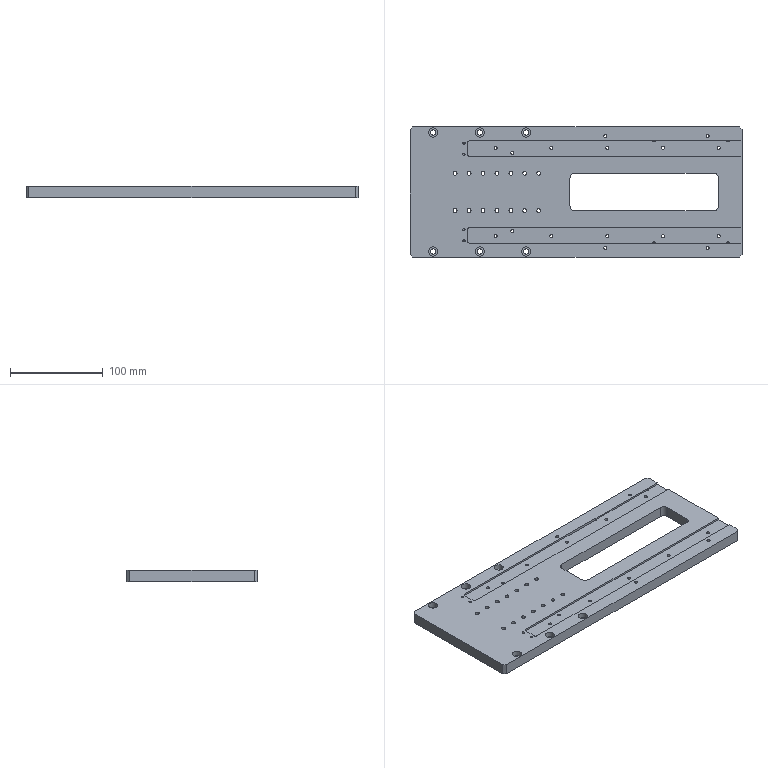NC program | NX | posted with a generic post | part box 357 x 140 x 12 mm
Lines 38 to 860 of 6551:
(ZLEVEL_PROFILE_1_1 , TOOL : D3)
N62 T16 M6
N64 G54
N66 G17 G0 G90 X-59.136 Y0.252 B0. C0. S9500 M3
N68 G43 Z30. H16
N70 Z1.5
N72 G94 G1 X-59.174 Y0.382 Z1.493 F1000.
N74 X-59.385 Y0.671 Z1.474
N76 X-59.692 Y0.856 Z1.455
N78 X-60.046 Y0.909 Z1.437
N80 X-60.394 Y0.82 Z1.418
N82 X-60.616 Y0.669 Z1.404
N84 X-60.836 Y0.36 Z1.384
N86 X-60.91 Y-0.012 Z1.364
N88 X-60.826 Y-0.381 Z1.344
N90 X-60.599 Y-0.685 Z1.324
N92 X-60.373 Y-0.83 Z1.31
N94 X-60.135 Y-0.9 Z1.297
N96 X-59.865 Z1.283
N98 X-59.564 Y-0.799 Z1.266
N100 X-59.315 Y-0.599 Z1.25
N102 X-59.17 Y-0.373 Z1.236
N104 X-59.099 Y-0.13 Z1.222
N106 X-59.098 Y0.123 Z1.209
N108 X-59.174 Y0.382 Z1.195
N110 X-59.385 Y0.671 Z1.176
N112 X-59.692 Y0.856 Z1.157
N114 X-60.046 Y0.909 Z1.139
N116 X-60.394 Y0.82 Z1.12
N118 X-60.616 Y0.669 Z1.106
N120 X-60.836 Y0.36 Z1.086
N122 X-60.91 Y-0.012 Z1.066
N124 X-60.826 Y-0.381 Z1.046
N126 X-60.599 Y-0.685 Z1.026
N128 X-60.373 Y-0.83 Z1.012
N130 X-60.135 Y-0.9 Z0.999
N132 X-59.865 Z0.985
N134 X-59.564 Y-0.799 Z0.968
N136 X-59.315 Y-0.599 Z0.952
N138 X-59.17 Y-0.373 Z0.938
N140 X-59.099 Y-0.13 Z0.924
N142 X-59.098 Y0.123 Z0.911
N144 X-59.174 Y0.382 Z0.897
N146 X-59.385 Y0.671 Z0.878
N148 X-59.692 Y0.856 Z0.859
N150 X-60.046 Y0.909 Z0.841
N152 X-60.394 Y0.82 Z0.822
N154 X-60.616 Y0.669 Z0.808
N156 X-60.836 Y0.36 Z0.788
N158 X-60.91 Y-0.012 Z0.768
N160 X-60.826 Y-0.381 Z0.748
N162 X-60.599 Y-0.685 Z0.728
N164 X-60.373 Y-0.83 Z0.714
N166 X-60.135 Y-0.9 Z0.701
N168 X-59.865 Z0.687
N170 X-59.564 Y-0.799 Z0.67
N172 X-59.315 Y-0.599 Z0.654
N174 X-59.17 Y-0.373 Z0.64
N176 X-59.099 Y-0.13 Z0.626
N178 X-59.098 Y0.123 Z0.613
N180 X-59.174 Y0.382 Z0.599
N182 X-59.385 Y0.671 Z0.58
N184 X-59.692 Y0.856 Z0.561
N186 X-60.046 Y0.909 Z0.543
N188 X-60.394 Y0.82 Z0.524
N190 X-60.616 Y0.669 Z0.51
N192 X-60.836 Y0.36 Z0.49
N194 X-60.91 Y-0.012 Z0.47
N196 X-60.826 Y-0.381 Z0.45
N198 X-60.599 Y-0.685 Z0.43
N200 X-60.373 Y-0.83 Z0.416
N202 X-60.135 Y-0.9 Z0.403
N204 X-59.865 Z0.389
N206 X-59.564 Y-0.799 Z0.372
N208 X-59.315 Y-0.599 Z0.356
N210 X-59.17 Y-0.373 Z0.341
N212 X-59.099 Y-0.13 Z0.328
N214 X-59.098 Y0.123 Z0.315
N216 X-59.174 Y0.382 Z0.301
N218 X-59.385 Y0.671 Z0.282
N220 X-59.692 Y0.856 Z0.263
N222 X-60.046 Y0.909 Z0.245
N224 X-60.394 Y0.82 Z0.226
N226 X-60.616 Y0.669 Z0.212
N228 X-60.836 Y0.36 Z0.192
N230 X-60.91 Y-0.012 Z0.172
N232 X-60.826 Y-0.381 Z0.152
N234 X-60.599 Y-0.685 Z0.132
N236 X-60.373 Y-0.83 Z0.118
N238 X-60.135 Y-0.9 Z0.105
N240 X-59.865 Z0.091
N242 X-59.564 Y-0.799 Z0.074
N244 X-59.315 Y-0.599 Z0.058
N246 X-59.17 Y-0.373 Z0.043
N248 X-59.099 Y-0.13 Z0.03
N250 X-59.098 Y0.123 Z0.017
N252 X-59.174 Y0.382 Z0.003
N254 X-59.385 Y0.671 Z-0.016
N256 X-59.692 Y0.856 Z-0.035
N258 X-60.046 Y0.909 Z-0.053
N260 X-60.394 Y0.82 Z-0.072
N262 X-60.616 Y0.669 Z-0.086
N264 X-60.836 Y0.36 Z-0.106
N266 X-60.91 Y-0.012 Z-0.126
N268 X-60.826 Y-0.381 Z-0.146
N270 X-60.599 Y-0.685 Z-0.166
N272 X-60.373 Y-0.83 Z-0.18
N274 X-60.135 Y-0.9 Z-0.193
N276 X-60. Z-0.2
N278 G3 X-59.1 Y0. R0.9 F1200.
N280 X-60. Y-0.9 R-0.9
N282 G1 X-59.878 Y-0.883 Z-0.204
N284 X-59.78 Y-0.863 Z-0.208
N286 X-59.649 Y-0.819 Z-0.213
N288 X-59.572 Y-0.784 Z-0.216
N290 X-59.471 Y-0.718 Z-0.22
N292 X-59.393 Y-0.652 Z-0.224
N294 X-59.299 Y-0.552 Z-0.229
N296 X-59.249 Y-0.482 Z-0.232
N298 X-59.181 Y-0.35 Z-0.237
N300 X-59.145 Y-0.251 Z-0.241
N302 X-59.115 Y-0.097 Z-0.247
N304 X-59.106 Y-0.001 Z-0.25
N306 X-59.113 Y0.087 Z-0.253
N308 X-59.117 Y0.131 Z-0.255
N310 X-59.123 Y0.171 Z-0.256
N312 X-59.145 Y0.25 Z-0.259
N314 X-59.201 Y0.394 Z-0.265
N316 X-59.241 Y0.469 Z-0.268
N318 X-59.293 Y0.543 Z-0.271
N320 X-59.319 Y0.579 Z-0.272
N322 X-59.344 Y0.604 Z-0.274
N324 X-59.394 Y0.653 Z-0.276
N326 X-59.512 Y0.746 Z-0.282
N328 X-59.588 Y0.791 Z-0.285
N330 X-59.718 Y0.847 Z-0.29
N332 X-59.813 Y0.872 Z-0.293
N334 X-59.95 Y0.89 Z-0.298
N336 X-60.052 Y0.889 Z-0.302
N338 X-60.196 Y0.87 Z-0.307
N340 X-60.287 Y0.846 Z-0.31
N342 X-60.408 Y0.792 Z-0.315
N344 X-60.5 Y0.737 Z-0.319
N346 X-60.621 Y0.639 Z-0.325
N348 X-60.688 Y0.571 Z-0.328
N350 X-60.739 Y0.498 Z-0.331
N352 X-60.764 Y0.462 Z-0.333
N354 X-60.783 Y0.427 Z-0.334
N356 X-60.817 Y0.356 Z-0.337
N358 X-60.853 Y0.256 Z-0.341
N360 X-60.876 Y0.175 Z-0.344
N362 X-60.885 Y0.114 Z-0.346
N364 X-60.89 Y-0.05 Z-0.352
N366 X-60.882 Y-0.137 Z-0.355
N368 X-60.849 Y-0.27 Z-0.36
N370 X-60.808 Y-0.376 Z-0.364
N372 X-60.732 Y-0.508 Z-0.369
N374 X-60.672 Y-0.588 Z-0.373
N376 X-60.606 Y-0.655 Z-0.376
N378 X-60.572 Y-0.687 Z-0.378
N380 X-60.542 Y-0.709 Z-0.379
N382 X-60.482 Y-0.751 Z-0.382
N384 X-60.353 Y-0.818 Z-0.387
N386 X-60.251 Y-0.855 Z-0.391
N388 X-60.126 Y-0.884 Z-0.395
N390 X-60. Y-0.9 Z-0.4
N392 X-59.878 Y-0.883 Z-0.404
N394 X-59.78 Y-0.863 Z-0.408
N396 X-59.649 Y-0.819 Z-0.413
N398 X-59.572 Y-0.784 Z-0.416
N400 X-59.472 Y-0.718 Z-0.42
N402 X-59.393 Y-0.652 Z-0.424
N404 X-59.299 Y-0.552 Z-0.429
N406 X-59.249 Y-0.482 Z-0.432
N408 X-59.181 Y-0.35 Z-0.437
N410 X-59.145 Y-0.251 Z-0.441
N412 X-59.115 Y-0.097 Z-0.447
N414 X-59.106 Y-0.001 Z-0.45
N416 X-59.113 Y0.087 Z-0.453
N418 X-59.117 Y0.131 Z-0.455
N420 X-59.124 Y0.171 Z-0.456
N422 X-59.145 Y0.25 Z-0.459
N424 X-59.201 Y0.394 Z-0.465
N426 X-59.241 Y0.469 Z-0.468
N428 X-59.293 Y0.543 Z-0.471
N430 X-59.319 Y0.579 Z-0.472
N432 X-59.344 Y0.604 Z-0.474
N434 X-59.394 Y0.653 Z-0.476
N436 X-59.512 Y0.746 Z-0.482
N438 X-59.588 Y0.791 Z-0.485
N440 X-59.718 Y0.847 Z-0.49
N442 X-59.813 Y0.872 Z-0.493
N444 X-59.95 Y0.89 Z-0.498
N446 X-60.052 Y0.889 Z-0.502
N448 X-60.196 Y0.87 Z-0.507
N450 X-60.287 Y0.846 Z-0.51
N452 X-60.408 Y0.792 Z-0.515
N454 X-60.5 Y0.737 Z-0.519
N456 X-60.621 Y0.639 Z-0.525
N458 X-60.688 Y0.571 Z-0.528
N460 X-60.739 Y0.498 Z-0.531
N462 X-60.764 Y0.462 Z-0.533
N464 X-60.783 Y0.427 Z-0.534
N466 X-60.817 Y0.356 Z-0.537
N468 X-60.853 Y0.256 Z-0.541
N470 X-60.876 Y0.175 Z-0.544
N472 X-60.885 Y0.114 Z-0.546
N474 X-60.89 Y-0.05 Z-0.552
N476 X-60.882 Y-0.137 Z-0.555
N478 X-60.849 Y-0.27 Z-0.56
N480 X-60.808 Y-0.376 Z-0.564
N482 X-60.732 Y-0.508 Z-0.569
N484 X-60.672 Y-0.588 Z-0.573
N486 X-60.606 Y-0.654 Z-0.576
N488 X-60.572 Y-0.687 Z-0.578
N490 X-60.542 Y-0.709 Z-0.579
N492 X-60.482 Y-0.751 Z-0.582
N494 X-60.353 Y-0.818 Z-0.587
N496 X-60.251 Y-0.855 Z-0.591
N498 X-60.126 Y-0.884 Z-0.595
N500 X-60. Y-0.9 Z-0.6
N502 X-59.878 Y-0.883 Z-0.604
N504 X-59.78 Y-0.863 Z-0.608
N506 X-59.649 Y-0.819 Z-0.613
N508 X-59.572 Y-0.784 Z-0.616
N510 X-59.472 Y-0.718 Z-0.62
N512 X-59.393 Y-0.652 Z-0.624
N514 X-59.299 Y-0.552 Z-0.629
N516 X-59.249 Y-0.482 Z-0.632
N518 X-59.181 Y-0.35 Z-0.637
N520 X-59.145 Y-0.251 Z-0.641
N522 X-59.115 Y-0.097 Z-0.647
N524 X-59.106 Y-0.001 Z-0.65
N526 X-59.113 Y0.087 Z-0.653
N528 X-59.117 Y0.131 Z-0.655
N530 X-59.124 Y0.171 Z-0.656
N532 X-59.145 Y0.25 Z-0.659
N534 X-59.201 Y0.394 Z-0.665
N536 X-59.241 Y0.469 Z-0.668
N538 X-59.293 Y0.542 Z-0.671
N540 X-59.319 Y0.579 Z-0.672
N542 X-59.344 Y0.604 Z-0.674
N544 X-59.394 Y0.653 Z-0.676
N546 X-59.512 Y0.746 Z-0.682
N548 X-59.588 Y0.791 Z-0.685
N550 X-59.718 Y0.847 Z-0.69
N552 X-59.813 Y0.872 Z-0.693
N554 X-59.95 Y0.889 Z-0.698
N556 X-60.052 Z-0.702
N558 X-60.196 Y0.87 Z-0.707
N560 X-60.287 Y0.846 Z-0.71
N562 X-60.408 Y0.792 Z-0.715
N564 X-60.5 Y0.737 Z-0.719
N566 X-60.621 Y0.639 Z-0.725
N568 X-60.688 Y0.571 Z-0.728
N570 X-60.739 Y0.498 Z-0.731
N572 X-60.764 Y0.462 Z-0.733
N574 X-60.783 Y0.427 Z-0.734
N576 X-60.817 Y0.356 Z-0.737
N578 X-60.853 Y0.256 Z-0.741
N580 X-60.876 Y0.175 Z-0.744
N582 X-60.885 Y0.114 Z-0.746
N584 X-60.889 Y-0.05 Z-0.752
N586 X-60.882 Y-0.137 Z-0.755
N588 X-60.849 Y-0.27 Z-0.76
N590 X-60.808 Y-0.376 Z-0.764
N592 X-60.732 Y-0.508 Z-0.769
N594 X-60.672 Y-0.588 Z-0.773
N596 X-60.606 Y-0.654 Z-0.776
N598 X-60.572 Y-0.687 Z-0.778
N600 X-60.542 Y-0.709 Z-0.779
N602 X-60.482 Y-0.751 Z-0.782
N604 X-60.354 Y-0.818 Z-0.787
N606 X-60.251 Y-0.855 Z-0.791
N608 X-60.126 Y-0.884 Z-0.795
N610 X-60. Y-0.9 Z-0.8
N612 X-59.879 Y-0.883 Z-0.804
N614 X-59.78 Y-0.863 Z-0.808
N616 X-59.649 Y-0.819 Z-0.813
N618 X-59.572 Y-0.784 Z-0.816
N620 X-59.472 Y-0.718 Z-0.82
N622 X-59.393 Y-0.652 Z-0.824
N624 X-59.299 Y-0.552 Z-0.829
N626 X-59.249 Y-0.482 Z-0.832
N628 X-59.181 Y-0.35 Z-0.837
N630 X-59.145 Y-0.251 Z-0.841
N632 X-59.115 Y-0.097 Z-0.847
N634 X-59.106 Y-0.001 Z-0.85
N636 X-59.113 Y0.087 Z-0.853
N638 X-59.117 Y0.131 Z-0.855
N640 X-59.124 Y0.171 Z-0.856
N642 X-59.145 Y0.25 Z-0.859
N644 X-59.201 Y0.394 Z-0.865
N646 X-59.241 Y0.469 Z-0.868
N648 X-59.293 Y0.545 Z-0.871
N650 X-59.321 Y0.581 Z-0.873
N652 X-59.345 Y0.605 Z-0.874
N654 X-59.394 Y0.653 Z-0.876
N656 X-59.513 Y0.747 Z-0.882
N658 X-59.588 Y0.791 Z-0.885
N660 X-59.718 Y0.847 Z-0.89
N662 X-59.813 Y0.872 Z-0.893
N664 X-59.95 Y0.889 Z-0.898
N666 X-60.052 Z-0.902
N668 X-60.196 Y0.87 Z-0.907
N670 X-60.287 Y0.846 Z-0.91
N672 X-60.408 Y0.792 Z-0.915
N674 X-60.5 Y0.737 Z-0.919
N676 X-60.621 Y0.639 Z-0.925
N678 X-60.688 Y0.571 Z-0.928
N680 X-60.739 Y0.498 Z-0.931
N682 X-60.764 Y0.462 Z-0.933
N684 X-60.783 Y0.427 Z-0.934
N686 X-60.817 Y0.356 Z-0.937
N688 X-60.853 Y0.256 Z-0.941
N690 X-60.875 Y0.176 Z-0.944
N692 X-60.885 Y0.114 Z-0.946
N694 X-60.889 Y-0.05 Z-0.952
N696 X-60.882 Y-0.137 Z-0.955
N698 X-60.849 Y-0.27 Z-0.96
N700 X-60.808 Y-0.376 Z-0.964
N702 X-60.732 Y-0.508 Z-0.969
N704 X-60.672 Y-0.588 Z-0.973
N706 X-60.606 Y-0.654 Z-0.976
N708 X-60.572 Y-0.687 Z-0.978
N710 X-60.542 Y-0.709 Z-0.979
N712 X-60.482 Y-0.751 Z-0.982
N714 X-60.354 Y-0.818 Z-0.987
N716 X-60.251 Y-0.855 Z-0.991
N718 X-60.126 Y-0.883 Z-0.995
N720 X-60. Y-0.9 Z-1.
N722 X-59.879 Y-0.883 Z-1.004
N724 X-59.78 Y-0.863 Z-1.008
N726 X-59.649 Y-0.819 Z-1.013
N728 X-59.572 Y-0.783 Z-1.016
N730 X-59.472 Y-0.718 Z-1.02
N732 X-59.393 Y-0.652 Z-1.024
N734 X-59.299 Y-0.552 Z-1.029
N736 X-59.249 Y-0.482 Z-1.032
N738 X-59.181 Y-0.35 Z-1.037
N740 X-59.145 Y-0.251 Z-1.041
N742 X-59.115 Y-0.097 Z-1.047
N744 X-59.106 Y-0.001 Z-1.05
N746 X-59.113 Y0.087 Z-1.053
N748 X-59.117 Y0.131 Z-1.055
N750 X-59.124 Y0.171 Z-1.056
N752 X-59.145 Y0.25 Z-1.059
N754 X-59.201 Y0.394 Z-1.065
N756 X-59.241 Y0.469 Z-1.068
N758 X-59.293 Y0.545 Z-1.071
N760 X-59.321 Y0.581 Z-1.073
N762 X-59.345 Y0.605 Z-1.074
N764 X-59.394 Y0.653 Z-1.076
N766 X-59.513 Y0.746 Z-1.082
N768 X-59.588 Y0.791 Z-1.085
N770 X-59.718 Y0.847 Z-1.09
N772 X-59.813 Y0.872 Z-1.093
N774 X-59.95 Y0.889 Z-1.098
N776 X-60.052 Z-1.102
N778 X-60.196 Y0.87 Z-1.107
N780 X-60.287 Y0.846 Z-1.11
N782 X-60.408 Y0.792 Z-1.115
N784 X-60.5 Y0.737 Z-1.119
N786 X-60.621 Y0.639 Z-1.125
N788 X-60.688 Y0.571 Z-1.128
N790 X-60.739 Y0.498 Z-1.131
N792 X-60.764 Y0.462 Z-1.133
N794 X-60.783 Y0.427 Z-1.134
N796 X-60.817 Y0.356 Z-1.137
N798 X-60.867 Y0.205 Z-1.143
N800 X-60.885 Y0.114 Z-1.146
N802 X-60.891 Y-0.037 Z-1.151
N804 X-60.882 Y-0.137 Z-1.155
N806 X-60.849 Y-0.27 Z-1.16
N808 X-60.808 Y-0.376 Z-1.164
N810 X-60.732 Y-0.508 Z-1.169
N812 X-60.672 Y-0.587 Z-1.173
N814 X-60.606 Y-0.654 Z-1.176
N816 X-60.572 Y-0.687 Z-1.178
N818 X-60.542 Y-0.709 Z-1.179
N820 X-60.482 Y-0.751 Z-1.182
N822 X-60.354 Y-0.817 Z-1.187
N824 X-60.251 Y-0.855 Z-1.191
N826 X-60.126 Y-0.883 Z-1.195
N828 X-60. Y-0.9 Z-1.2
N830 X-59.879 Y-0.883 Z-1.204
N832 X-59.78 Y-0.863 Z-1.208
N834 X-59.649 Y-0.819 Z-1.213
N836 X-59.572 Y-0.783 Z-1.216
N838 X-59.472 Y-0.718 Z-1.22
N840 X-59.393 Y-0.652 Z-1.224
N842 X-59.299 Y-0.552 Z-1.229
N844 X-59.249 Y-0.482 Z-1.232
N846 X-59.181 Y-0.35 Z-1.237
N848 X-59.145 Y-0.251 Z-1.241
N850 X-59.115 Y-0.098 Z-1.247
N852 X-59.106 Y-0.001 Z-1.25
N854 X-59.113 Y0.087 Z-1.253
N856 X-59.117 Y0.131 Z-1.255
N858 X-59.124 Y0.171 Z-1.256
N860 X-59.145 Y0.25 Z-1.259
N862 X-59.2 Y0.394 Z-1.265
N864 X-59.241 Y0.469 Z-1.268
N866 X-59.293 Y0.545 Z-1.271
N868 X-59.321 Y0.581 Z-1.273
N870 X-59.345 Y0.605 Z-1.274
N872 X-59.394 Y0.653 Z-1.276
N874 X-59.513 Y0.746 Z-1.282
N876 X-59.588 Y0.791 Z-1.285
N878 X-59.718 Y0.847 Z-1.29
N880 X-59.813 Y0.872 Z-1.293
N882 X-59.95 Y0.889 Z-1.298
N884 X-60.052 Z-1.302
N886 X-60.196 Y0.87 Z-1.307
N888 X-60.287 Y0.846 Z-1.31
N890 X-60.408 Y0.792 Z-1.315
N892 X-60.5 Y0.737 Z-1.319
N894 X-60.621 Y0.639 Z-1.325
N896 X-60.688 Y0.571 Z-1.328
N898 X-60.739 Y0.499 Z-1.331
N900 X-60.764 Y0.462 Z-1.333
N902 X-60.783 Y0.427 Z-1.334
N904 X-60.817 Y0.356 Z-1.337
N906 X-60.867 Y0.206 Z-1.343
N908 X-60.885 Y0.114 Z-1.346
N910 X-60.891 Y-0.037 Z-1.351
N912 X-60.882 Y-0.137 Z-1.355
N914 X-60.849 Y-0.27 Z-1.36
N916 X-60.808 Y-0.376 Z-1.364
N918 X-60.732 Y-0.508 Z-1.369
N920 X-60.672 Y-0.587 Z-1.373
N922 X-60.606 Y-0.654 Z-1.376
N924 X-60.572 Y-0.687 Z-1.378
N926 X-60.542 Y-0.708 Z-1.379
N928 X-60.482 Y-0.751 Z-1.382
N930 X-60.354 Y-0.817 Z-1.387
N932 X-60.251 Y-0.855 Z-1.391
N934 X-60.126 Y-0.883 Z-1.395
N936 X-60. Y-0.9 Z-1.4
N938 X-59.879 Y-0.883 Z-1.404
N940 X-59.78 Y-0.863 Z-1.408
N942 X-59.65 Y-0.819 Z-1.413
N944 X-59.572 Y-0.783 Z-1.416
N946 X-59.472 Y-0.718 Z-1.42
N948 X-59.393 Y-0.652 Z-1.424
N950 X-59.299 Y-0.552 Z-1.429
N952 X-59.249 Y-0.482 Z-1.432
N954 X-59.181 Y-0.35 Z-1.437
N956 X-59.145 Y-0.251 Z-1.441
N958 X-59.115 Y-0.098 Z-1.447
N960 X-59.106 Y-0.001 Z-1.45
N962 X-59.113 Y0.087 Z-1.453
N964 X-59.117 Y0.131 Z-1.455
N966 X-59.124 Y0.171 Z-1.456
N968 X-59.145 Y0.25 Z-1.459
N970 X-59.2 Y0.394 Z-1.465
N972 X-59.241 Y0.469 Z-1.468
N974 X-59.293 Y0.545 Z-1.471
N976 X-59.321 Y0.581 Z-1.473
N978 X-59.345 Y0.605 Z-1.474
N980 X-59.394 Y0.653 Z-1.476
N982 X-59.513 Y0.746 Z-1.482
N984 X-59.588 Y0.791 Z-1.485
N986 X-59.718 Y0.847 Z-1.49
N988 X-59.813 Y0.872 Z-1.493
N990 X-59.95 Y0.889 Z-1.498
N992 X-60.052 Z-1.502
N994 X-60.196 Y0.87 Z-1.507
N996 X-60.287 Y0.846 Z-1.51
N998 X-60.408 Y0.792 Z-1.515
N1000 X-60.5 Y0.737 Z-1.519
N1002 X-60.621 Y0.639 Z-1.525
N1004 X-60.688 Y0.571 Z-1.528
N1006 X-60.739 Y0.499 Z-1.531
N1008 X-60.764 Y0.462 Z-1.533
N1010 X-60.783 Y0.428 Z-1.534
N1012 X-60.817 Y0.356 Z-1.537
N1014 X-60.867 Y0.206 Z-1.543
N1016 X-60.884 Y0.114 Z-1.546
N1018 X-60.891 Y-0.037 Z-1.551
N1020 X-60.882 Y-0.137 Z-1.555
N1022 X-60.849 Y-0.27 Z-1.56
N1024 X-60.808 Y-0.376 Z-1.564
N1026 X-60.732 Y-0.507 Z-1.569
N1028 X-60.672 Y-0.587 Z-1.573
N1030 X-60.606 Y-0.654 Z-1.576
N1032 X-60.572 Y-0.687 Z-1.578
N1034 X-60.542 Y-0.708 Z-1.579
N1036 X-60.482 Y-0.751 Z-1.582
N1038 X-60.398 Y-0.798 Z-1.585
N1040 X-60.321 Y-0.834 Z-1.588
N1042 X-60.251 Y-0.855 Z-1.591
N1044 X-60.126 Y-0.883 Z-1.595
N1046 X-60. Y-0.9 Z-1.6
N1048 X-59.879 Y-0.883 Z-1.604
N1050 X-59.78 Y-0.863 Z-1.608
N1052 X-59.65 Y-0.819 Z-1.613
N1054 X-59.572 Y-0.783 Z-1.616
N1056 X-59.472 Y-0.718 Z-1.62
N1058 X-59.393 Y-0.652 Z-1.624
N1060 X-59.299 Y-0.552 Z-1.629
N1062 X-59.249 Y-0.482 Z-1.632
N1064 X-59.181 Y-0.35 Z-1.637
N1066 X-59.145 Y-0.251 Z-1.641
N1068 X-59.115 Y-0.098 Z-1.646
N1070 X-59.106 Y-0.001 Z-1.65
N1072 X-59.113 Y0.087 Z-1.653
N1074 X-59.117 Y0.131 Z-1.655
N1076 X-59.124 Y0.171 Z-1.656
N1078 X-59.145 Y0.25 Z-1.659
N1080 X-59.2 Y0.394 Z-1.665
N1082 X-59.241 Y0.469 Z-1.668
N1084 X-59.293 Y0.544 Z-1.671
N1086 X-59.321 Y0.581 Z-1.673
N1088 X-59.345 Y0.605 Z-1.674
N1090 X-59.394 Y0.653 Z-1.676
N1092 X-59.513 Y0.746 Z-1.682
N1094 X-59.588 Y0.791 Z-1.685
N1096 X-59.718 Y0.847 Z-1.69
N1098 X-59.813 Y0.872 Z-1.693
N1100 X-59.95 Y0.89 Z-1.698
N1102 X-60.052 Y0.889 Z-1.702
N1104 X-60.198 Y0.869 Z-1.707
N1106 X-60.287 Y0.846 Z-1.71
N1108 X-60.408 Y0.792 Z-1.715
N1110 X-60.5 Y0.737 Z-1.719
N1112 X-60.621 Y0.639 Z-1.725
N1114 X-60.688 Y0.571 Z-1.728
N1116 X-60.739 Y0.499 Z-1.731
N1118 X-60.764 Y0.462 Z-1.733
N1120 X-60.783 Y0.428 Z-1.734
N1122 X-60.817 Y0.356 Z-1.737
N1124 X-60.867 Y0.206 Z-1.743
N1126 X-60.884 Y0.114 Z-1.746
N1128 X-60.89 Y-0.037 Z-1.751
N1130 X-60.882 Y-0.137 Z-1.755
N1132 X-60.849 Y-0.27 Z-1.76
N1134 X-60.807 Y-0.376 Z-1.764
N1136 X-60.732 Y-0.507 Z-1.769
N1138 X-60.672 Y-0.587 Z-1.773
N1140 X-60.606 Y-0.654 Z-1.776
N1142 X-60.572 Y-0.687 Z-1.778
N1144 X-60.542 Y-0.708 Z-1.779
N1146 X-60.482 Y-0.751 Z-1.782
N1148 X-60.398 Y-0.797 Z-1.785
N1150 X-60.321 Y-0.833 Z-1.788
N1152 X-60.251 Y-0.855 Z-1.791
N1154 X-60.126 Y-0.883 Z-1.795
N1156 X-60. Y-0.9 Z-1.8
N1158 X-59.879 Y-0.883 Z-1.804
N1160 X-59.78 Y-0.863 Z-1.808
N1162 X-59.65 Y-0.819 Z-1.813
N1164 X-59.572 Y-0.783 Z-1.816
N1166 X-59.472 Y-0.718 Z-1.82
N1168 X-59.393 Y-0.652 Z-1.824
N1170 X-59.3 Y-0.552 Z-1.829
N1172 X-59.249 Y-0.482 Z-1.832
N1174 X-59.201 Y-0.395 Z-1.835
N1176 X-59.166 Y-0.318 Z-1.838
N1178 X-59.145 Y-0.251 Z-1.841
N1180 X-59.114 Y-0.082 Z-1.847
N1182 X-59.106 Y-0.001 Z-1.85
N1184 X-59.113 Y0.087 Z-1.853
N1186 X-59.117 Y0.131 Z-1.855
N1188 X-59.124 Y0.171 Z-1.856
N1190 X-59.145 Y0.25 Z-1.859
N1192 X-59.2 Y0.394 Z-1.865
N1194 X-59.241 Y0.469 Z-1.868
N1196 X-59.293 Y0.544 Z-1.871
N1198 X-59.321 Y0.581 Z-1.873
N1200 X-59.345 Y0.605 Z-1.874
N1202 X-59.394 Y0.653 Z-1.876
N1204 X-59.513 Y0.746 Z-1.882
N1206 X-59.588 Y0.791 Z-1.885
N1208 X-59.718 Y0.846 Z-1.89
N1210 X-59.813 Y0.872 Z-1.893
N1212 X-59.95 Y0.89 Z-1.898
N1214 X-60.052 Y0.889 Z-1.902
N1216 X-60.198 Y0.869 Z-1.907
N1218 X-60.287 Y0.845 Z-1.91
N1220 X-60.408 Y0.792 Z-1.915
N1222 X-60.5 Y0.737 Z-1.919
N1224 X-60.62 Y0.639 Z-1.925
N1226 X-60.688 Y0.571 Z-1.928
N1228 X-60.739 Y0.499 Z-1.931
N1230 X-60.764 Y0.462 Z-1.933
N1232 X-60.783 Y0.428 Z-1.934
N1234 X-60.817 Y0.356 Z-1.937
N1236 X-60.867 Y0.206 Z-1.943
N1238 X-60.884 Y0.114 Z-1.946
N1240 X-60.89 Y-0.037 Z-1.951
N1242 X-60.882 Y-0.137 Z-1.955
N1244 X-60.849 Y-0.27 Z-1.96
N1246 X-60.807 Y-0.376 Z-1.964
N1248 X-60.732 Y-0.507 Z-1.969
N1250 X-60.672 Y-0.587 Z-1.973
N1252 X-60.606 Y-0.654 Z-1.976
N1254 X-60.572 Y-0.687 Z-1.978
N1256 X-60.542 Y-0.708 Z-1.979
N1258 X-60.482 Y-0.751 Z-1.982
N1260 X-60.398 Y-0.797 Z-1.985
N1262 X-60.321 Y-0.833 Z-1.988
N1264 X-60.251 Y-0.855 Z-1.991
N1266 X-60.126 Y-0.883 Z-1.995
N1268 X-60. Y-0.9 Z-2.
N1270 X-59.879 Y-0.883 Z-2.004
N1272 X-59.78 Y-0.863 Z-2.008
N1274 X-59.65 Y-0.819 Z-2.013
N1276 X-59.572 Y-0.783 Z-2.016
N1278 X-59.472 Y-0.718 Z-2.02
N1280 X-59.393 Y-0.652 Z-2.024
N1282 X-59.3 Y-0.552 Z-2.029
N1284 X-59.249 Y-0.482 Z-2.032
N1286 X-59.201 Y-0.395 Z-2.035
N1288 X-59.165 Y-0.319 Z-2.038
N1290 X-59.145 Y-0.251 Z-2.041
N1292 X-59.113 Y-0.077 Z-2.047
N1294 X-59.106 Y-0.001 Z-2.05
N1296 X-59.113 Y0.087 Z-2.053
N1298 X-59.117 Y0.132 Z-2.055
N1300 X-59.124 Y0.171 Z-2.056
N1302 X-59.145 Y0.25 Z-2.059
N1304 X-59.201 Y0.394 Z-2.065
N1306 X-59.241 Y0.469 Z-2.068
N1308 X-59.293 Y0.544 Z-2.071
N1310 X-59.321 Y0.581 Z-2.073
N1312 X-59.345 Y0.605 Z-2.074
N1314 X-59.394 Y0.653 Z-2.076
N1316 X-59.513 Y0.746 Z-2.082
N1318 X-59.588 Y0.791 Z-2.085
N1320 X-59.718 Y0.846 Z-2.09
N1322 X-59.813 Y0.872 Z-2.093
N1324 X-59.95 Y0.89 Z-2.098
N1326 X-60.052 Y0.889 Z-2.102
N1328 X-60.198 Y0.869 Z-2.107
N1330 X-60.287 Y0.845 Z-2.11
N1332 X-60.408 Y0.792 Z-2.115
N1334 X-60.5 Y0.737 Z-2.119
N1336 X-60.62 Y0.639 Z-2.125
N1338 X-60.688 Y0.571 Z-2.128
N1340 X-60.738 Y0.499 Z-2.131
N1342 X-60.764 Y0.462 Z-2.133
N1344 X-60.784 Y0.428 Z-2.134
N1346 X-60.817 Y0.356 Z-2.137
N1348 X-60.868 Y0.202 Z-2.143
N1350 X-60.884 Y0.114 Z-2.146
N1352 X-60.89 Y-0.038 Z-2.151
N1354 X-60.882 Y-0.137 Z-2.155
N1356 X-60.862 Y-0.226 Z-2.158
N1358 X-60.839 Y-0.307 Z-2.161
N1360 X-60.807 Y-0.376 Z-2.164
N1362 X-60.721 Y-0.523 Z-2.17
N1364 X-60.672 Y-0.587 Z-2.173
N1366 X-60.605 Y-0.655 Z-2.176
N1368 X-60.571 Y-0.688 Z-2.178
N1370 X-60.541 Y-0.709 Z-2.179
N1372 X-60.482 Y-0.751 Z-2.182
N1374 X-60.398 Y-0.797 Z-2.185
N1376 X-60.321 Y-0.833 Z-2.188
N1378 X-60.251 Y-0.855 Z-2.191
N1380 X-60.126 Y-0.883 Z-2.195
N1382 X-60. Y-0.9 Z-2.2
N1384 X-59.879 Y-0.883 Z-2.204
N1386 X-59.78 Y-0.863 Z-2.208
N1388 X-59.65 Y-0.819 Z-2.213
N1390 X-59.572 Y-0.783 Z-2.216
N1392 X-59.472 Y-0.718 Z-2.22
N1394 X-59.393 Y-0.652 Z-2.224
N1396 X-59.3 Y-0.552 Z-2.229
N1398 X-59.249 Y-0.482 Z-2.232
N1400 X-59.201 Y-0.395 Z-2.235
N1402 X-59.165 Y-0.319 Z-2.238
N1404 X-59.145 Y-0.251 Z-2.241
N1406 X-59.113 Y-0.077 Z-2.247
N1408 X-59.106 Y-0.001 Z-2.25
N1410 X-59.113 Y0.087 Z-2.253
N1412 X-59.117 Y0.131 Z-2.255
N1414 X-59.124 Y0.171 Z-2.256
N1416 X-59.145 Y0.25 Z-2.259
N1418 X-59.201 Y0.394 Z-2.265
N1420 X-59.241 Y0.469 Z-2.268
N1422 X-59.293 Y0.544 Z-2.271
N1424 X-59.321 Y0.581 Z-2.273
N1426 X-59.345 Y0.605 Z-2.274
N1428 X-59.394 Y0.653 Z-2.276
N1430 X-59.512 Y0.746 Z-2.282
N1432 X-59.588 Y0.791 Z-2.285
N1434 X-59.718 Y0.846 Z-2.29
N1436 X-59.813 Y0.872 Z-2.293
N1438 X-59.95 Y0.89 Z-2.298
N1440 X-60.052 Y0.889 Z-2.302
N1442 X-60.198 Y0.869 Z-2.307
N1444 X-60.287 Y0.845 Z-2.31
N1446 X-60.408 Y0.792 Z-2.315
N1448 X-60.5 Y0.737 Z-2.319
N1450 X-60.62 Y0.639 Z-2.325
N1452 X-60.688 Y0.571 Z-2.328
N1454 X-60.738 Y0.499 Z-2.331
N1456 X-60.764 Y0.462 Z-2.333
N1458 X-60.784 Y0.428 Z-2.334
N1460 X-60.817 Y0.356 Z-2.337
N1462 X-60.868 Y0.202 Z-2.343
N1464 X-60.884 Y0.114 Z-2.346
N1466 X-60.89 Y-0.038 Z-2.351
N1468 X-60.882 Y-0.137 Z-2.355
N1470 X-60.862 Y-0.226 Z-2.358
N1472 X-60.839 Y-0.307 Z-2.361
N1474 X-60.807 Y-0.376 Z-2.364
N1476 X-60.721 Y-0.523 Z-2.37
N1478 X-60.672 Y-0.587 Z-2.373
N1480 X-60.605 Y-0.655 Z-2.376
N1482 X-60.571 Y-0.688 Z-2.378
N1484 X-60.541 Y-0.709 Z-2.379
N1486 X-60.482 Y-0.751 Z-2.382
N1488 X-60.398 Y-0.797 Z-2.385
N1490 X-60.321 Y-0.833 Z-2.388
N1492 X-60.251 Y-0.855 Z-2.391
N1494 X-60.126 Y-0.883 Z-2.395
N1496 X-60. Y-0.9 Z-2.4
N1498 X-59.879 Y-0.883 Z-2.404
N1500 X-59.78 Y-0.863 Z-2.408
N1502 X-59.65 Y-0.819 Z-2.413
N1504 X-59.572 Y-0.783 Z-2.416
N1506 X-59.472 Y-0.718 Z-2.42
N1508 X-59.393 Y-0.652 Z-2.424
N1510 X-59.3 Y-0.552 Z-2.429
N1512 X-59.249 Y-0.482 Z-2.432
N1514 X-59.202 Y-0.395 Z-2.435
N1516 X-59.165 Y-0.319 Z-2.438
N1518 X-59.145 Y-0.251 Z-2.441
N1520 X-59.113 Y-0.077 Z-2.447
N1522 X-59.106 Y-0.001 Z-2.45
N1524 X-59.113 Y0.087 Z-2.453
N1526 X-59.117 Y0.131 Z-2.455
N1528 X-59.124 Y0.171 Z-2.456
N1530 X-59.145 Y0.25 Z-2.459
N1532 X-59.201 Y0.394 Z-2.465
N1534 X-59.241 Y0.469 Z-2.468
N1536 X-59.293 Y0.544 Z-2.471
N1538 X-59.321 Y0.581 Z-2.473
N1540 X-59.345 Y0.605 Z-2.474
N1542 X-59.394 Y0.653 Z-2.476
N1544 X-59.512 Y0.746 Z-2.482
N1546 X-59.588 Y0.791 Z-2.485
N1548 X-59.718 Y0.846 Z-2.49
N1550 X-59.813 Y0.872 Z-2.493
N1552 X-59.95 Y0.89 Z-2.498
N1554 X-60.052 Y0.889 Z-2.502
N1556 X-60.198 Y0.869 Z-2.507
N1558 X-60.287 Y0.845 Z-2.51
N1560 X-60.408 Y0.792 Z-2.515
N1562 X-60.5 Y0.737 Z-2.519
N1564 X-60.62 Y0.639 Z-2.525
N1566 X-60.688 Y0.571 Z-2.528
N1568 X-60.738 Y0.499 Z-2.531
N1570 X-60.764 Y0.462 Z-2.533
N1572 X-60.784 Y0.428 Z-2.534
N1574 X-60.817 Y0.356 Z-2.537
N1576 X-60.868 Y0.202 Z-2.543
N1578 X-60.884 Y0.114 Z-2.546
N1580 X-60.89 Y-0.038 Z-2.551
N1582 X-60.882 Y-0.137 Z-2.555
N1584 X-60.862 Y-0.226 Z-2.558
N1586 X-60.839 Y-0.307 Z-2.561
N1588 X-60.807 Y-0.376 Z-2.564
N1590 X-60.721 Y-0.523 Z-2.57
N1592 X-60.672 Y-0.587 Z-2.573
N1594 X-60.605 Y-0.654 Z-2.576
N1596 X-60.571 Y-0.687 Z-2.578
N1598 X-60.541 Y-0.709 Z-2.579
N1600 X-60.482 Y-0.751 Z-2.582
N1602 X-60.398 Y-0.797 Z-2.585
N1604 X-60.321 Y-0.833 Z-2.588
N1606 X-60.251 Y-0.855 Z-2.591
N1608 X-60.126 Y-0.883 Z-2.595
N1610 X-60. Y-0.9 Z-2.6
N1612 X-59.879 Y-0.883 Z-2.604
N1614 X-59.78 Y-0.863 Z-2.608
N1616 X-59.65 Y-0.819 Z-2.613
N1618 X-59.572 Y-0.783 Z-2.616
N1620 X-59.472 Y-0.718 Z-2.62
N1622 X-59.393 Y-0.652 Z-2.624
N1624 X-59.3 Y-0.553 Z-2.629
N1626 X-59.249 Y-0.482 Z-2.632
N1628 X-59.202 Y-0.395 Z-2.635
N1630 X-59.166 Y-0.319 Z-2.638
N1632 X-59.145 Y-0.251 Z-2.641
N1634 X-59.113 Y-0.078 Z-2.647
N1636 X-59.106 Y-0.001 Z-2.65
N1638 X-59.113 Y0.087 Z-2.653
N1640 X-59.117 Y0.131 Z-2.655
N1642 X-59.124 Y0.171 Z-2.656
N1644 X-59.145 Y0.25 Z-2.659
N1646 X-59.201 Y0.394 Z-2.665
N1648 X-59.241 Y0.469 Z-2.668
N1650 X-59.293 Y0.544 Z-2.671
N1652 X-59.321 Y0.581 Z-2.673
N1654 X-59.345 Y0.605 Z-2.674
N1656 X-59.394 Y0.653 Z-2.676
N1658 X-59.512 Y0.746 Z-2.682
N1660 X-59.588 Y0.791 Z-2.685
N1662 X-59.718 Y0.846 Z-2.69
N1664 X-59.813 Y0.872 Z-2.693
N1666 X-59.95 Y0.89 Z-2.698
N1668 X-60.052 Y0.889 Z-2.702
N1670 X-60.198 Y0.869 Z-2.707
N1672 X-60.287 Y0.845 Z-2.71
N1674 X-60.408 Y0.792 Z-2.715
N1676 X-60.5 Y0.737 Z-2.719
N1678 X-60.62 Y0.639 Z-2.725
N1680 X-60.688 Y0.571 Z-2.728
N1682 X-60.738 Y0.499 Z-2.731
N1684 X-60.763 Y0.462 Z-2.733
N1686 X-60.784 Y0.428 Z-2.734
N1688 X-60.817 Y0.356 Z-2.737
N1690 X-60.868 Y0.202 Z-2.743
N1692 X-60.884 Y0.114 Z-2.746
N1694 X-60.89 Y-0.038 Z-2.751
N1696 X-60.882 Y-0.137 Z-2.755
N1698 X-60.862 Y-0.226 Z-2.758
N1700 X-60.839 Y-0.307 Z-2.761